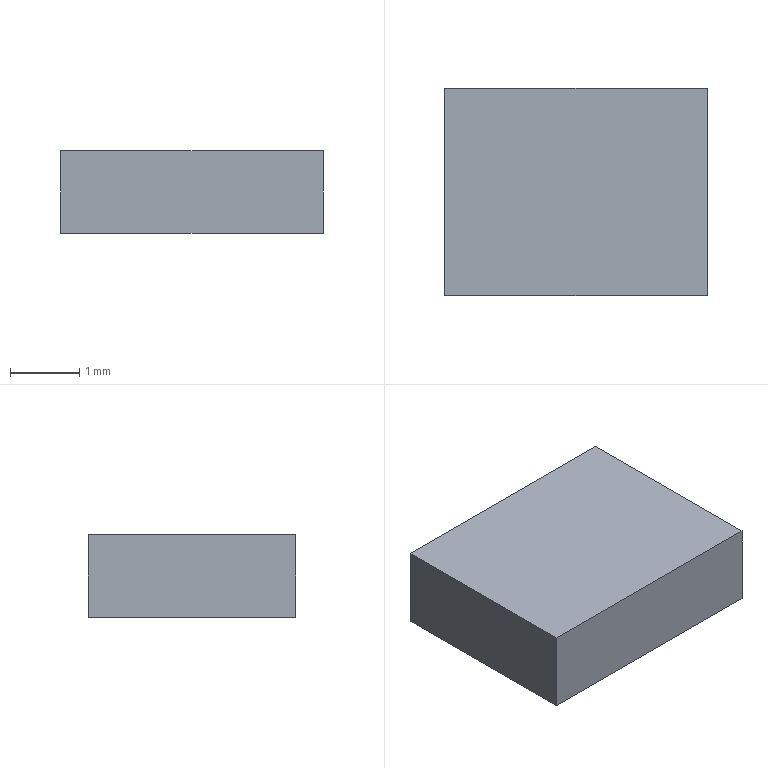Part | STEP file | 1 solid | 9 faces | box 3.8 x 3 x 1.2 mm | volume 13.052 mm3 | plane 7 | cylinder 2 | commonest cylinder face diameters 2 x2
STEP:
#1=CARTESIAN_POINT('',(0.,0.,0.));
#2=DIRECTION('',(0.,0.,1.));
#3=DIRECTION('',(1.,0.,0.));
#4=AXIS2_PLACEMENT_3D('',#1,#2,#3);
#5=CARTESIAN_POINT('',(1.,0.,-1.));
#6=VERTEX_POINT('',#5);
#7=CARTESIAN_POINT('',(-1.,0.,-1.));
#8=VERTEX_POINT('',#7);
#9=CARTESIAN_POINT('',(0.,0.,-1.));
#10=DIRECTION('',(0.,0.,-1.));
#11=DIRECTION('',(1.,0.,0.));
#12=AXIS2_PLACEMENT_3D('',#9,#10,#11);
#13=CIRCLE('',#12,1.);
#14=EDGE_CURVE('',#6,#8,#13,.T.);
#15=ORIENTED_EDGE('',*,*,#14,.T.);
#16=CARTESIAN_POINT('',(-1.,0.,-1.2));
#17=VERTEX_POINT('',#16);
#18=CARTESIAN_POINT('',(-1.,0.,-1.2));
#19=DIRECTION('',(0.,0.,1.));
#20=VECTOR('',#19,0.2);
#21=LINE('',#18,#20);
#22=EDGE_CURVE('',#17,#8,#21,.T.);
#23=ORIENTED_EDGE('',*,*,#22,.F.);
#24=CARTESIAN_POINT('',(1.,0.,-1.2));
#25=VERTEX_POINT('',#24);
#26=CARTESIAN_POINT('',(0.,0.,-1.2));
#27=DIRECTION('',(0.,0.,1.));
#28=DIRECTION('',(-1.,0.,0.));
#29=AXIS2_PLACEMENT_3D('',#26,#27,#28);
#30=CIRCLE('',#29,1.);
#31=EDGE_CURVE('',#17,#25,#30,.T.);
#32=ORIENTED_EDGE('',*,*,#31,.T.);
#33=CARTESIAN_POINT('',(1.,0.,-1.2));
#34=DIRECTION('',(0.,0.,1.));
#35=VECTOR('',#34,0.2);
#36=LINE('',#33,#35);
#37=EDGE_CURVE('',#25,#6,#36,.T.);
#38=ORIENTED_EDGE('',*,*,#37,.T.);
#39=EDGE_LOOP('',(#15,#23,#32,#38));
#40=FACE_OUTER_BOUND('',#39,.F.);
#41=CARTESIAN_POINT('',(0.,0.,-1.));
#42=DIRECTION('',(0.,0.,-1.));
#43=DIRECTION('',(-1.,0.,0.));
#44=AXIS2_PLACEMENT_3D('',#41,#42,#43);
#45=CYLINDRICAL_SURFACE('',#44,1.);
#46=ADVANCED_FACE('',(#40),#45,.F.);
#47=CARTESIAN_POINT('',(0.,0.,-1.));
#48=DIRECTION('',(0.,0.,-1.));
#49=DIRECTION('',(-1.,0.,0.));
#50=AXIS2_PLACEMENT_3D('',#47,#48,#49);
#51=CIRCLE('',#50,1.);
#52=EDGE_CURVE('',#8,#6,#51,.T.);
#53=ORIENTED_EDGE('',*,*,#52,.F.);
#54=ORIENTED_EDGE('',*,*,#14,.F.);
#55=EDGE_LOOP('',(#53,#54));
#56=FACE_OUTER_BOUND('',#55,.F.);
#57=CARTESIAN_POINT('',(0.,0.,-1.));
#58=DIRECTION('',(0.,0.,-1.));
#59=DIRECTION('',(-1.,0.,0.));
#60=AXIS2_PLACEMENT_3D('',#57,#58,#59);
#61=PLANE('',#60);
#62=ADVANCED_FACE('',(#56),#61,.T.);
#63=ORIENTED_EDGE('',*,*,#37,.F.);
#64=CARTESIAN_POINT('',(0.,0.,-1.2));
#65=DIRECTION('',(0.,0.,1.));
#66=DIRECTION('',(1.,0.,0.));
#67=AXIS2_PLACEMENT_3D('',#64,#65,#66);
#68=CIRCLE('',#67,1.);
#69=EDGE_CURVE('',#25,#17,#68,.T.);
#70=ORIENTED_EDGE('',*,*,#69,.T.);
#71=ORIENTED_EDGE('',*,*,#22,.T.);
#72=ORIENTED_EDGE('',*,*,#52,.T.);
#73=EDGE_LOOP('',(#63,#70,#71,#72));
#74=FACE_OUTER_BOUND('',#73,.F.);
#75=CARTESIAN_POINT('',(0.,0.,-1.));
#76=DIRECTION('',(0.,0.,-1.));
#77=DIRECTION('',(-1.,0.,0.));
#78=AXIS2_PLACEMENT_3D('',#75,#76,#77);
#79=CYLINDRICAL_SURFACE('',#78,1.);
#80=ADVANCED_FACE('',(#74),#79,.F.);
#81=CARTESIAN_POINT('',(-1.9,-1.5,-1.2));
#82=VERTEX_POINT('',#81);
#83=CARTESIAN_POINT('',(-1.9,1.5,-1.2));
#84=VERTEX_POINT('',#83);
#85=CARTESIAN_POINT('',(-1.9,-1.5,-1.2));
#86=DIRECTION('',(0.,1.,0.));
#87=VECTOR('',#86,3.);
#88=LINE('',#85,#87);
#89=EDGE_CURVE('',#82,#84,#88,.T.);
#90=ORIENTED_EDGE('',*,*,#89,.F.);
#91=CARTESIAN_POINT('',(1.9,-1.5,-1.2));
#92=VERTEX_POINT('',#91);
#93=CARTESIAN_POINT('',(1.9,-1.5,-1.2));
#94=DIRECTION('',(-1.,0.,0.));
#95=VECTOR('',#94,3.8);
#96=LINE('',#93,#95);
#97=EDGE_CURVE('',#92,#82,#96,.T.);
#98=ORIENTED_EDGE('',*,*,#97,.F.);
#99=CARTESIAN_POINT('',(1.9,1.5,-1.2));
#100=VERTEX_POINT('',#99);
#101=CARTESIAN_POINT('',(1.9,1.5,-1.2));
#102=DIRECTION('',(0.,-1.,0.));
#103=VECTOR('',#102,3.);
#104=LINE('',#101,#103);
#105=EDGE_CURVE('',#100,#92,#104,.T.);
#106=ORIENTED_EDGE('',*,*,#105,.F.);
#107=CARTESIAN_POINT('',(-1.9,1.5,-1.2));
#108=DIRECTION('',(1.,0.,0.));
#109=VECTOR('',#108,3.8);
#110=LINE('',#107,#109);
#111=EDGE_CURVE('',#84,#100,#110,.T.);
#112=ORIENTED_EDGE('',*,*,#111,.F.);
#113=EDGE_LOOP('',(#90,#98,#106,#112));
#114=FACE_OUTER_BOUND('',#113,.F.);
#115=ORIENTED_EDGE('',*,*,#69,.F.);
#116=ORIENTED_EDGE('',*,*,#31,.F.);
#117=EDGE_LOOP('',(#115,#116));
#118=FACE_BOUND('',#117,.F.);
#119=CARTESIAN_POINT('',(0.,0.,-1.2));
#120=DIRECTION('',(0.,0.,-1.));
#121=DIRECTION('',(-1.,0.,0.));
#122=AXIS2_PLACEMENT_3D('',#119,#120,#121);
#123=PLANE('',#122);
#124=ADVANCED_FACE('',(#114,#118),#123,.T.);
#125=CARTESIAN_POINT('',(-1.9,-1.5,0.));
#126=VERTEX_POINT('',#125);
#127=CARTESIAN_POINT('',(-1.9,1.5,0.));
#128=VERTEX_POINT('',#127);
#129=CARTESIAN_POINT('',(-1.9,-1.5,0.));
#130=DIRECTION('',(0.,1.,0.));
#131=VECTOR('',#130,3.);
#132=LINE('',#129,#131);
#133=EDGE_CURVE('',#126,#128,#132,.T.);
#134=ORIENTED_EDGE('',*,*,#133,.F.);
#135=CARTESIAN_POINT('',(-1.9,-1.5,0.));
#136=DIRECTION('',(0.,0.,-1.));
#137=VECTOR('',#136,1.2);
#138=LINE('',#135,#137);
#139=EDGE_CURVE('',#126,#82,#138,.T.);
#140=ORIENTED_EDGE('',*,*,#139,.T.);
#141=ORIENTED_EDGE('',*,*,#89,.T.);
#142=CARTESIAN_POINT('',(-1.9,1.5,0.));
#143=DIRECTION('',(0.,0.,-1.));
#144=VECTOR('',#143,1.2);
#145=LINE('',#142,#144);
#146=EDGE_CURVE('',#128,#84,#145,.T.);
#147=ORIENTED_EDGE('',*,*,#146,.F.);
#148=EDGE_LOOP('',(#134,#140,#141,#147));
#149=FACE_OUTER_BOUND('',#148,.F.);
#150=CARTESIAN_POINT('',(-1.9,1.5,-1.2));
#151=DIRECTION('',(-1.,0.,0.));
#152=DIRECTION('',(0.,-1.,0.));
#153=AXIS2_PLACEMENT_3D('',#150,#151,#152);
#154=PLANE('',#153);
#155=ADVANCED_FACE('',(#149),#154,.T.);
#156=ORIENTED_EDGE('',*,*,#133,.T.);
#157=CARTESIAN_POINT('',(1.9,1.5,0.));
#158=VERTEX_POINT('',#157);
#159=CARTESIAN_POINT('',(-1.9,1.5,0.));
#160=DIRECTION('',(1.,0.,0.));
#161=VECTOR('',#160,3.8);
#162=LINE('',#159,#161);
#163=EDGE_CURVE('',#128,#158,#162,.T.);
#164=ORIENTED_EDGE('',*,*,#163,.T.);
#165=CARTESIAN_POINT('',(1.9,-1.5,0.));
#166=VERTEX_POINT('',#165);
#167=CARTESIAN_POINT('',(1.9,1.5,0.));
#168=DIRECTION('',(0.,-1.,0.));
#169=VECTOR('',#168,3.);
#170=LINE('',#167,#169);
#171=EDGE_CURVE('',#158,#166,#170,.T.);
#172=ORIENTED_EDGE('',*,*,#171,.T.);
#173=CARTESIAN_POINT('',(1.9,-1.5,0.));
#174=DIRECTION('',(-1.,0.,0.));
#175=VECTOR('',#174,3.8);
#176=LINE('',#173,#175);
#177=EDGE_CURVE('',#166,#126,#176,.T.);
#178=ORIENTED_EDGE('',*,*,#177,.T.);
#179=EDGE_LOOP('',(#156,#164,#172,#178));
#180=FACE_OUTER_BOUND('',#179,.F.);
#181=CARTESIAN_POINT('',(0.,0.,0.));
#182=DIRECTION('',(0.,0.,-1.));
#183=DIRECTION('',(-1.,0.,0.));
#184=AXIS2_PLACEMENT_3D('',#181,#182,#183);
#185=PLANE('',#184);
#186=ADVANCED_FACE('',(#180),#185,.F.);
#187=ORIENTED_EDGE('',*,*,#163,.F.);
#188=ORIENTED_EDGE('',*,*,#146,.T.);
#189=ORIENTED_EDGE('',*,*,#111,.T.);
#190=CARTESIAN_POINT('',(1.9,1.5,0.));
#191=DIRECTION('',(0.,0.,-1.));
#192=VECTOR('',#191,1.2);
#193=LINE('',#190,#192);
#194=EDGE_CURVE('',#158,#100,#193,.T.);
#195=ORIENTED_EDGE('',*,*,#194,.F.);
#196=EDGE_LOOP('',(#187,#188,#189,#195));
#197=FACE_OUTER_BOUND('',#196,.F.);
#198=CARTESIAN_POINT('',(1.9,1.5,-1.2));
#199=DIRECTION('',(0.,1.,0.));
#200=DIRECTION('',(-1.,0.,0.));
#201=AXIS2_PLACEMENT_3D('',#198,#199,#200);
#202=PLANE('',#201);
#203=ADVANCED_FACE('',(#197),#202,.T.);
#204=ORIENTED_EDGE('',*,*,#171,.F.);
#205=ORIENTED_EDGE('',*,*,#194,.T.);
#206=ORIENTED_EDGE('',*,*,#105,.T.);
#207=CARTESIAN_POINT('',(1.9,-1.5,0.));
#208=DIRECTION('',(0.,0.,-1.));
#209=VECTOR('',#208,1.2);
#210=LINE('',#207,#209);
#211=EDGE_CURVE('',#166,#92,#210,.T.);
#212=ORIENTED_EDGE('',*,*,#211,.F.);
#213=EDGE_LOOP('',(#204,#205,#206,#212));
#214=FACE_OUTER_BOUND('',#213,.F.);
#215=CARTESIAN_POINT('',(1.9,1.5,-1.2));
#216=DIRECTION('',(1.,0.,0.));
#217=DIRECTION('',(0.,1.,0.));
#218=AXIS2_PLACEMENT_3D('',#215,#216,#217);
#219=PLANE('',#218);
#220=ADVANCED_FACE('',(#214),#219,.T.);
#221=ORIENTED_EDGE('',*,*,#177,.F.);
#222=ORIENTED_EDGE('',*,*,#211,.T.);
#223=ORIENTED_EDGE('',*,*,#97,.T.);
#224=ORIENTED_EDGE('',*,*,#139,.F.);
#225=EDGE_LOOP('',(#221,#222,#223,#224));
#226=FACE_OUTER_BOUND('',#225,.F.);
#227=CARTESIAN_POINT('',(1.9,-1.5,-1.2));
#228=DIRECTION('',(0.,-1.,0.));
#229=DIRECTION('',(1.,0.,0.));
#230=AXIS2_PLACEMENT_3D('',#227,#228,#229);
#231=PLANE('',#230);
#232=ADVANCED_FACE('',(#226),#231,.T.);
#233=CLOSED_SHELL('',(#46,#62,#80,#124,#155,#186,#203,#220,#232));
#234=MANIFOLD_SOLID_BREP('',#233);
#235=(LENGTH_UNIT()NAMED_UNIT(*)SI_UNIT(.MILLI.,.METRE.));
#236=UNCERTAINTY_MEASURE_WITH_UNIT(LENGTH_MEASURE(0.0004988),#235,'','');
#237=(NAMED_UNIT(*)PLANE_ANGLE_UNIT()SI_UNIT($,.RADIAN.));
#238=PLANE_ANGLE_MEASURE_WITH_UNIT(PLANE_ANGLE_MEASURE(0.01745),#237);
#239=(CONVERSION_BASED_UNIT('DEGREE',#238)NAMED_UNIT(*)PLANE_ANGLE_UNIT());
#240=(NAMED_UNIT(*)SI_UNIT($,.STERADIAN.)SOLID_ANGLE_UNIT());
#241=(GEOMETRIC_REPRESENTATION_CONTEXT(3)GLOBAL_UNCERTAINTY_ASSIGNED_CONTEXT((#236))GLOBAL_UNIT_ASSIGNED_CONTEXT((#235,#239,#240))REPRESENTATION_CONTEXT('',''));
#242=ADVANCED_BREP_SHAPE_REPRESENTATION('',(#4,#234),#241);